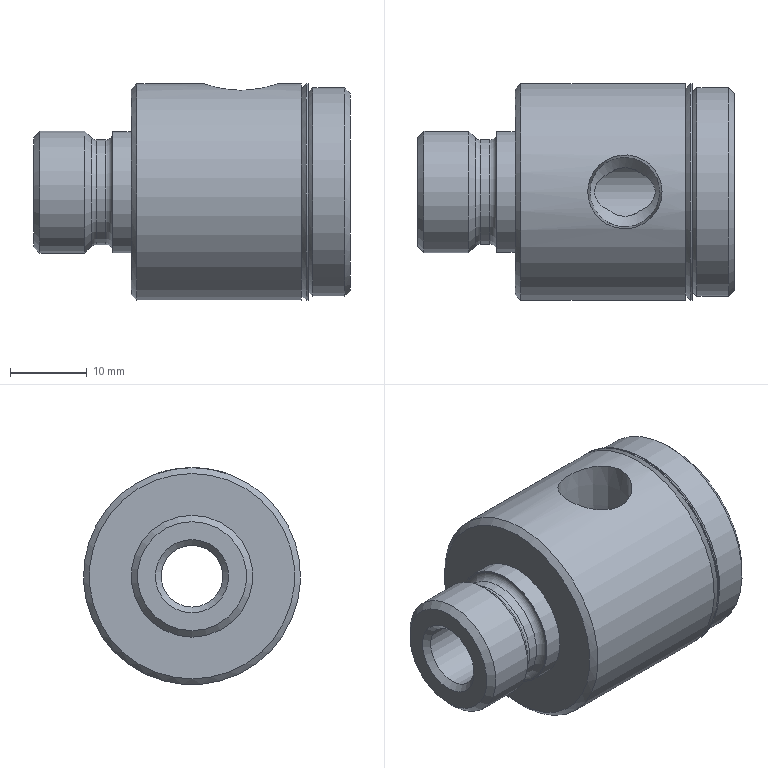Part | NX | features solid 2 | 1 solid | 30 faces | box 41.275 x 28.27 x 28.27 mm | volume 17100 mm3 | cone 11 | cylinder 10 | plane 6 | torus 3 | commonest cylinder face diameters 6.35 x2 28.27 x2 8.026 x1 13.678 x1 15.812 x1 15.875 x1
STEP:
#1=CARTESIAN_POINT('',(34.861,0.,14.135));
#2=VERTEX_POINT('',#1);
#3=CARTESIAN_POINT('',(34.861,0.,0.));
#4=DIRECTION('',(-1.,0.,0.));
#5=DIRECTION('',(0.,0.,1.));
#6=AXIS2_PLACEMENT_3D('',#3,#4,#5);
#7=CIRCLE('',#6,14.135);
#8=EDGE_CURVE('',#2,#2,#7,.T.);
#9=ORIENTED_EDGE('',*,*,#8,.F.);
#10=EDGE_LOOP('',(#9));
#11=FACE_BOUND('',#10,.T.);
#12=CARTESIAN_POINT('',(34.861,0.,13.449));
#13=VERTEX_POINT('',#12);
#14=CARTESIAN_POINT('',(34.861,0.,0.));
#15=DIRECTION('',(-1.,0.,0.));
#16=DIRECTION('',(0.,0.,1.));
#17=AXIS2_PLACEMENT_3D('',#14,#15,#16);
#18=CIRCLE('',#17,13.449);
#19=EDGE_CURVE('',#13,#13,#18,.T.);
#20=ORIENTED_EDGE('',*,*,#19,.T.);
#21=EDGE_LOOP('',(#20));
#22=FACE_BOUND('',#21,.T.);
#23=CARTESIAN_POINT('',(34.861,14.135,0.));
#24=DIRECTION('',(1.,0.,0.));
#25=DIRECTION('',(0.,0.,-1.));
#26=AXIS2_PLACEMENT_3D('',#23,#24,#25);
#27=PLANE('',#26);
#28=ADVANCED_FACE('',(#11,#22),#27,.T.);
#29=CARTESIAN_POINT('',(35.623,0.,12.846));
#30=VERTEX_POINT('',#29);
#31=CARTESIAN_POINT('',(35.623,0.,0.));
#32=DIRECTION('',(-1.,0.,0.));
#33=DIRECTION('',(0.,0.,1.));
#34=AXIS2_PLACEMENT_3D('',#31,#32,#33);
#35=CIRCLE('',#34,12.846);
#36=EDGE_CURVE('',#30,#30,#35,.T.);
#37=ORIENTED_EDGE('',*,*,#36,.T.);
#38=EDGE_LOOP('',(#37));
#39=FACE_BOUND('',#38,.T.);
#40=CARTESIAN_POINT('',(35.242,0.,12.846));
#41=VERTEX_POINT('',#40);
#42=CARTESIAN_POINT('',(35.242,0.,0.));
#43=DIRECTION('',(-1.,0.,0.));
#44=DIRECTION('',(0.,0.,1.));
#45=AXIS2_PLACEMENT_3D('',#42,#43,#44);
#46=CIRCLE('',#45,12.846);
#47=EDGE_CURVE('',#41,#41,#46,.T.);
#48=ORIENTED_EDGE('',*,*,#47,.F.);
#49=EDGE_LOOP('',(#48));
#50=FACE_BOUND('',#49,.T.);
#51=CARTESIAN_POINT('',(41.275,0.,0.));
#52=DIRECTION('',(-1.,0.,0.));
#53=DIRECTION('',(0.,0.,1.));
#54=AXIS2_PLACEMENT_3D('',#51,#52,#53);
#55=CYLINDRICAL_SURFACE('',#54,12.846);
#56=ADVANCED_FACE('',(#39,#50),#55,.T.);
#57=CARTESIAN_POINT('',(7.513,0.,7.099));
#58=VERTEX_POINT('',#57);
#59=CARTESIAN_POINT('',(7.513,0.,0.));
#60=DIRECTION('',(-1.,0.,0.));
#61=DIRECTION('',(0.,0.,1.));
#62=AXIS2_PLACEMENT_3D('',#59,#60,#61);
#63=CIRCLE('',#62,7.099);
#64=EDGE_CURVE('',#58,#58,#63,.T.);
#65=ORIENTED_EDGE('',*,*,#64,.T.);
#66=EDGE_LOOP('',(#65));
#67=FACE_BOUND('',#66,.T.);
#68=CARTESIAN_POINT('',(6.673,0.,7.938));
#69=VERTEX_POINT('',#68);
#70=CARTESIAN_POINT('',(6.673,0.,0.));
#71=DIRECTION('',(-1.,0.,0.));
#72=DIRECTION('',(0.,0.,1.));
#73=AXIS2_PLACEMENT_3D('',#70,#71,#72);
#74=CIRCLE('',#73,7.938);
#75=EDGE_CURVE('',#69,#69,#74,.T.);
#76=ORIENTED_EDGE('',*,*,#75,.F.);
#77=EDGE_LOOP('',(#76));
#78=FACE_BOUND('',#77,.T.);
#79=CARTESIAN_POINT('',(6.673,0.,0.));
#80=DIRECTION('',(-1.,0.,0.));
#81=DIRECTION('',(0.,0.,1.));
#82=AXIS2_PLACEMENT_3D('',#79,#80,#81);
#83=CONICAL_SURFACE('',#82,7.938,0.7846);
#84=ADVANCED_FACE('',(#67,#78),#83,.T.);
#85=ORIENTED_EDGE('',*,*,#64,.F.);
#86=EDGE_LOOP('',(#85));
#87=FACE_BOUND('',#86,.T.);
#88=CARTESIAN_POINT('',(8.141,0.,6.839));
#89=VERTEX_POINT('',#88);
#90=CARTESIAN_POINT('',(8.141,0.,0.));
#91=DIRECTION('',(-1.,0.,0.));
#92=DIRECTION('',(0.,0.,1.));
#93=AXIS2_PLACEMENT_3D('',#90,#91,#92);
#94=CIRCLE('',#93,6.839);
#95=EDGE_CURVE('',#89,#89,#94,.T.);
#96=ORIENTED_EDGE('',*,*,#95,.T.);
#97=EDGE_LOOP('',(#96));
#98=FACE_BOUND('',#97,.T.);
#99=CARTESIAN_POINT('',(8.141,0.,0.));
#100=DIRECTION('',(-1.,0.,0.));
#101=DIRECTION('',(0.,0.,1.));
#102=AXIS2_PLACEMENT_3D('',#99,#100,#101);
#103=TOROIDAL_SURFACE('',#102,7.728,0.889);
#104=ADVANCED_FACE('',(#87,#98),#103,.F.);
#105=CARTESIAN_POINT('',(9.423,0.,6.839));
#106=VERTEX_POINT('',#105);
#107=CARTESIAN_POINT('',(9.423,0.,0.));
#108=DIRECTION('',(-1.,0.,0.));
#109=DIRECTION('',(0.,0.,1.));
#110=AXIS2_PLACEMENT_3D('',#107,#108,#109);
#111=CIRCLE('',#110,6.839);
#112=EDGE_CURVE('',#106,#106,#111,.T.);
#113=ORIENTED_EDGE('',*,*,#112,.T.);
#114=EDGE_LOOP('',(#113));
#115=FACE_BOUND('',#114,.T.);
#116=ORIENTED_EDGE('',*,*,#95,.F.);
#117=EDGE_LOOP('',(#116));
#118=FACE_BOUND('',#117,.T.);
#119=CARTESIAN_POINT('',(12.7,0.,0.));
#120=DIRECTION('',(-1.,0.,0.));
#121=DIRECTION('',(0.,0.,1.));
#122=AXIS2_PLACEMENT_3D('',#119,#120,#121);
#123=CYLINDRICAL_SURFACE('',#122,6.839);
#124=ADVANCED_FACE('',(#115,#118),#123,.T.);
#125=ORIENTED_EDGE('',*,*,#112,.F.);
#126=EDGE_LOOP('',(#125));
#127=FACE_BOUND('',#126,.T.);
#128=CARTESIAN_POINT('',(10.312,0.,7.728));
#129=VERTEX_POINT('',#128);
#130=CARTESIAN_POINT('',(10.312,0.,0.));
#131=DIRECTION('',(-1.,0.,0.));
#132=DIRECTION('',(0.,0.,1.));
#133=AXIS2_PLACEMENT_3D('',#130,#131,#132);
#134=CIRCLE('',#133,7.728);
#135=EDGE_CURVE('',#129,#129,#134,.T.);
#136=ORIENTED_EDGE('',*,*,#135,.T.);
#137=EDGE_LOOP('',(#136));
#138=FACE_BOUND('',#137,.T.);
#139=CARTESIAN_POINT('',(9.423,0.,0.));
#140=DIRECTION('',(-1.,0.,0.));
#141=DIRECTION('',(0.,0.,1.));
#142=AXIS2_PLACEMENT_3D('',#139,#140,#141);
#143=TOROIDAL_SURFACE('',#142,7.728,0.889);
#144=ADVANCED_FACE('',(#127,#138),#143,.F.);
#145=CARTESIAN_POINT('',(10.312,0.,7.906));
#146=VERTEX_POINT('',#145);
#147=CARTESIAN_POINT('',(10.312,0.,0.));
#148=DIRECTION('',(-1.,0.,0.));
#149=DIRECTION('',(0.,0.,1.));
#150=AXIS2_PLACEMENT_3D('',#147,#148,#149);
#151=CIRCLE('',#150,7.906);
#152=EDGE_CURVE('',#146,#146,#151,.T.);
#153=ORIENTED_EDGE('',*,*,#152,.T.);
#154=EDGE_LOOP('',(#153));
#155=FACE_BOUND('',#154,.T.);
#156=ORIENTED_EDGE('',*,*,#135,.F.);
#157=EDGE_LOOP('',(#156));
#158=FACE_BOUND('',#157,.T.);
#159=CARTESIAN_POINT('',(10.312,7.728,0.));
#160=DIRECTION('',(-1.,0.,0.));
#161=DIRECTION('',(0.,0.,1.));
#162=AXIS2_PLACEMENT_3D('',#159,#160,#161);
#163=PLANE('',#162);
#164=ADVANCED_FACE('',(#155,#158),#163,.T.);
#165=CARTESIAN_POINT('',(12.7,0.,7.906));
#166=VERTEX_POINT('',#165);
#167=CARTESIAN_POINT('',(12.7,0.,0.));
#168=DIRECTION('',(-1.,0.,0.));
#169=DIRECTION('',(0.,0.,1.));
#170=AXIS2_PLACEMENT_3D('',#167,#168,#169);
#171=CIRCLE('',#170,7.906);
#172=EDGE_CURVE('',#166,#166,#171,.F.);
#173=ORIENTED_EDGE('',*,*,#172,.F.);
#174=EDGE_LOOP('',(#173));
#175=FACE_BOUND('',#174,.T.);
#176=ORIENTED_EDGE('',*,*,#152,.F.);
#177=EDGE_LOOP('',(#176));
#178=FACE_BOUND('',#177,.T.);
#179=CARTESIAN_POINT('',(12.7,0.,0.));
#180=DIRECTION('',(-1.,0.,0.));
#181=DIRECTION('',(0.,0.,1.));
#182=AXIS2_PLACEMENT_3D('',#179,#180,#181);
#183=CYLINDRICAL_SURFACE('',#182,7.906);
#184=ADVANCED_FACE('',(#175,#178),#183,.T.);
#185=CARTESIAN_POINT('',(0.,0.,-4.775));
#186=VERTEX_POINT('',#185);
#187=CARTESIAN_POINT('',(0.,0.,0.));
#188=DIRECTION('',(1.,0.,0.));
#189=DIRECTION('',(0.,0.,-1.));
#190=AXIS2_PLACEMENT_3D('',#187,#188,#189);
#191=CIRCLE('',#190,4.775);
#192=EDGE_CURVE('',#186,#186,#191,.T.);
#193=ORIENTED_EDGE('',*,*,#192,.T.);
#194=EDGE_LOOP('',(#193));
#195=FACE_BOUND('',#194,.T.);
#196=CARTESIAN_POINT('',(0.,0.,7.098));
#197=VERTEX_POINT('',#196);
#198=CARTESIAN_POINT('',(0.,0.,0.));
#199=DIRECTION('',(-1.,0.,0.));
#200=DIRECTION('',(0.,0.,1.));
#201=AXIS2_PLACEMENT_3D('',#198,#199,#200);
#202=CIRCLE('',#201,7.098);
#203=EDGE_CURVE('',#197,#197,#202,.T.);
#204=ORIENTED_EDGE('',*,*,#203,.T.);
#205=EDGE_LOOP('',(#204));
#206=FACE_BOUND('',#205,.T.);
#207=CARTESIAN_POINT('',(0.,0.,0.));
#208=DIRECTION('',(-1.,0.,0.));
#209=DIRECTION('',(0.,0.,1.));
#210=AXIS2_PLACEMENT_3D('',#207,#208,#209);
#211=PLANE('',#210);
#212=ADVANCED_FACE('',(#195,#206),#211,.T.);
#213=CARTESIAN_POINT('',(0.8395,0.,7.938));
#214=VERTEX_POINT('',#213);
#215=CARTESIAN_POINT('',(0.8395,0.,0.));
#216=DIRECTION('',(-1.,0.,0.));
#217=DIRECTION('',(0.,0.,1.));
#218=AXIS2_PLACEMENT_3D('',#215,#216,#217);
#219=CIRCLE('',#218,7.938);
#220=EDGE_CURVE('',#214,#214,#219,.T.);
#221=ORIENTED_EDGE('',*,*,#220,.T.);
#222=EDGE_LOOP('',(#221));
#223=FACE_BOUND('',#222,.T.);
#224=ORIENTED_EDGE('',*,*,#203,.F.);
#225=EDGE_LOOP('',(#224));
#226=FACE_BOUND('',#225,.T.);
#227=CARTESIAN_POINT('',(0.,0.,0.));
#228=DIRECTION('',(1.,0.,0.));
#229=DIRECTION('',(0.,0.,-1.));
#230=AXIS2_PLACEMENT_3D('',#227,#228,#229);
#231=CONICAL_SURFACE('',#230,7.098,0.7854);
#232=ADVANCED_FACE('',(#223,#226),#231,.T.);
#233=ORIENTED_EDGE('',*,*,#75,.T.);
#234=EDGE_LOOP('',(#233));
#235=FACE_BOUND('',#234,.T.);
#236=ORIENTED_EDGE('',*,*,#220,.F.);
#237=EDGE_LOOP('',(#236));
#238=FACE_BOUND('',#237,.T.);
#239=CARTESIAN_POINT('',(12.7,0.,0.));
#240=DIRECTION('',(-1.,0.,0.));
#241=DIRECTION('',(0.,0.,1.));
#242=AXIS2_PLACEMENT_3D('',#239,#240,#241);
#243=CYLINDRICAL_SURFACE('',#242,7.938);
#244=ADVANCED_FACE('',(#235,#238),#243,.T.);
#245=CARTESIAN_POINT('',(36.386,0.,13.608));
#246=VERTEX_POINT('',#245);
#247=CARTESIAN_POINT('',(36.386,0.,0.));
#248=DIRECTION('',(-1.,0.,0.));
#249=DIRECTION('',(0.,0.,1.));
#250=AXIS2_PLACEMENT_3D('',#247,#248,#249);
#251=CIRCLE('',#250,13.608);
#252=EDGE_CURVE('',#246,#246,#251,.T.);
#253=ORIENTED_EDGE('',*,*,#252,.T.);
#254=EDGE_LOOP('',(#253));
#255=FACE_BOUND('',#254,.T.);
#256=ORIENTED_EDGE('',*,*,#36,.F.);
#257=EDGE_LOOP('',(#256));
#258=FACE_BOUND('',#257,.T.);
#259=CARTESIAN_POINT('',(35.623,0.,0.));
#260=DIRECTION('',(1.,0.,0.));
#261=DIRECTION('',(0.,0.,-1.));
#262=AXIS2_PLACEMENT_3D('',#259,#260,#261);
#263=CONICAL_SURFACE('',#262,12.846,0.7854);
#264=ADVANCED_FACE('',(#255,#258),#263,.T.);
#265=CARTESIAN_POINT('',(40.513,0.,13.608));
#266=VERTEX_POINT('',#265);
#267=CARTESIAN_POINT('',(40.513,0.,0.));
#268=DIRECTION('',(-1.,0.,0.));
#269=DIRECTION('',(0.,0.,1.));
#270=AXIS2_PLACEMENT_3D('',#267,#268,#269);
#271=CIRCLE('',#270,13.608);
#272=EDGE_CURVE('',#266,#266,#271,.T.);
#273=ORIENTED_EDGE('',*,*,#272,.T.);
#274=EDGE_LOOP('',(#273));
#275=FACE_BOUND('',#274,.T.);
#276=ORIENTED_EDGE('',*,*,#252,.F.);
#277=EDGE_LOOP('',(#276));
#278=FACE_BOUND('',#277,.T.);
#279=CARTESIAN_POINT('',(41.275,0.,0.));
#280=DIRECTION('',(-1.,0.,0.));
#281=DIRECTION('',(0.,0.,1.));
#282=AXIS2_PLACEMENT_3D('',#279,#280,#281);
#283=CYLINDRICAL_SURFACE('',#282,13.608);
#284=ADVANCED_FACE('',(#275,#278),#283,.T.);
#285=CARTESIAN_POINT('',(41.275,0.,12.846));
#286=VERTEX_POINT('',#285);
#287=CARTESIAN_POINT('',(41.275,0.,0.));
#288=DIRECTION('',(-1.,0.,0.));
#289=DIRECTION('',(0.,0.,1.));
#290=AXIS2_PLACEMENT_3D('',#287,#288,#289);
#291=CIRCLE('',#290,12.846);
#292=EDGE_CURVE('',#286,#286,#291,.T.);
#293=ORIENTED_EDGE('',*,*,#292,.T.);
#294=EDGE_LOOP('',(#293));
#295=FACE_BOUND('',#294,.T.);
#296=ORIENTED_EDGE('',*,*,#272,.F.);
#297=EDGE_LOOP('',(#296));
#298=FACE_BOUND('',#297,.T.);
#299=CARTESIAN_POINT('',(40.513,0.,0.));
#300=DIRECTION('',(-1.,0.,0.));
#301=DIRECTION('',(0.,0.,1.));
#302=AXIS2_PLACEMENT_3D('',#299,#300,#301);
#303=CONICAL_SURFACE('',#302,13.608,0.7854);
#304=ADVANCED_FACE('',(#295,#298),#303,.T.);
#305=CARTESIAN_POINT('',(41.275,0.,-4.013));
#306=VERTEX_POINT('',#305);
#307=CARTESIAN_POINT('',(41.275,0.,0.));
#308=DIRECTION('',(1.,0.,0.));
#309=DIRECTION('',(0.,0.,-1.));
#310=AXIS2_PLACEMENT_3D('',#307,#308,#309);
#311=CIRCLE('',#310,4.013);
#312=EDGE_CURVE('',#306,#306,#311,.T.);
#313=ORIENTED_EDGE('',*,*,#312,.F.);
#314=EDGE_LOOP('',(#313));
#315=FACE_BOUND('',#314,.T.);
#316=ORIENTED_EDGE('',*,*,#292,.F.);
#317=EDGE_LOOP('',(#316));
#318=FACE_BOUND('',#317,.T.);
#319=CARTESIAN_POINT('',(41.275,12.846,0.));
#320=DIRECTION('',(1.,0.,0.));
#321=DIRECTION('',(0.,0.,-1.));
#322=AXIS2_PLACEMENT_3D('',#319,#320,#321);
#323=PLANE('',#322);
#324=ADVANCED_FACE('',(#315,#318),#323,.T.);
#325=ORIENTED_EDGE('',*,*,#172,.T.);
#326=EDGE_LOOP('',(#325));
#327=FACE_BOUND('',#326,.T.);
#328=CARTESIAN_POINT('',(12.7,0.,13.373));
#329=VERTEX_POINT('',#328);
#330=CARTESIAN_POINT('',(12.7,0.,0.));
#331=DIRECTION('',(-1.,0.,0.));
#332=DIRECTION('',(0.,0.,1.));
#333=AXIS2_PLACEMENT_3D('',#330,#331,#332);
#334=CIRCLE('',#333,13.373);
#335=EDGE_CURVE('',#329,#329,#334,.T.);
#336=ORIENTED_EDGE('',*,*,#335,.T.);
#337=EDGE_LOOP('',(#336));
#338=FACE_BOUND('',#337,.T.);
#339=CARTESIAN_POINT('',(12.7,0.,0.));
#340=DIRECTION('',(-1.,0.,0.));
#341=DIRECTION('',(0.,0.,1.));
#342=AXIS2_PLACEMENT_3D('',#339,#340,#341);
#343=PLANE('',#342);
#344=ADVANCED_FACE('',(#327,#338),#343,.T.);
#345=CARTESIAN_POINT('',(13.462,0.,14.135));
#346=VERTEX_POINT('',#345);
#347=CARTESIAN_POINT('',(13.462,0.,0.));
#348=DIRECTION('',(-1.,0.,0.));
#349=DIRECTION('',(0.,0.,1.));
#350=AXIS2_PLACEMENT_3D('',#347,#348,#349);
#351=CIRCLE('',#350,14.135);
#352=EDGE_CURVE('',#346,#346,#351,.T.);
#353=ORIENTED_EDGE('',*,*,#352,.T.);
#354=EDGE_LOOP('',(#353));
#355=FACE_BOUND('',#354,.T.);
#356=ORIENTED_EDGE('',*,*,#335,.F.);
#357=EDGE_LOOP('',(#356));
#358=FACE_BOUND('',#357,.T.);
#359=CARTESIAN_POINT('',(12.7,0.,0.));
#360=DIRECTION('',(1.,0.,0.));
#361=DIRECTION('',(0.,0.,-1.));
#362=AXIS2_PLACEMENT_3D('',#359,#360,#361);
#363=CONICAL_SURFACE('',#362,13.373,0.7854);
#364=ADVANCED_FACE('',(#355,#358),#363,.T.);
#365=CARTESIAN_POINT('',(23.692,-3.513,13.691));
#366=VERTEX_POINT('',#365);
#367=CARTESIAN_POINT('',(21.636,-0.1674,14.34));
#368=CARTESIAN_POINT('',(23.337,-3.897,13.683));
#369=CARTESIAN_POINT('',(27.171,-5.326,13.076));
#370=CARTESIAN_POINT('',(30.898,-3.664,13.762));
#371=CARTESIAN_POINT('',(32.366,0.1695,14.34));
#372=CARTESIAN_POINT('',(30.663,3.895,13.684));
#373=CARTESIAN_POINT('',(26.836,5.328,13.075));
#374=CARTESIAN_POINT('',(23.097,3.659,13.763));
#375=CARTESIAN_POINT('',(21.636,-0.1674,14.34));
#376=CARTESIAN_POINT('',(23.337,-3.897,13.683));
#377=CARTESIAN_POINT('',(27.171,-5.326,13.076));
#378=B_SPLINE_CURVE_WITH_KNOTS('',3,(#367,#368,#369,#370,#371,#372,#373,#374,#375,#376,#377),.UNSPECIFIED.,.T.,.F.,(1,1,1,1,1,1,1,1,1,1,1,1,1,1,1),(-0.0114,-0.007602,-0.003801,0.,0.003801,0.007602,0.0114,0.0152,0.01901,0.02281,0.02661,0.03041,0.03421,0.03801,0.04181),.UNSPECIFIED.);
#379=EDGE_CURVE('',#366,#366,#378,.T.);
#380=ORIENTED_EDGE('',*,*,#379,.F.);
#381=EDGE_LOOP('',(#380));
#382=FACE_BOUND('',#381,.T.);
#383=ORIENTED_EDGE('',*,*,#8,.T.);
#384=EDGE_LOOP('',(#383));
#385=FACE_BOUND('',#384,.T.);
#386=ORIENTED_EDGE('',*,*,#352,.F.);
#387=EDGE_LOOP('',(#386));
#388=FACE_BOUND('',#387,.T.);
#389=CARTESIAN_POINT('',(41.275,0.,0.));
#390=DIRECTION('',(-1.,0.,0.));
#391=DIRECTION('',(0.,0.,1.));
#392=AXIS2_PLACEMENT_3D('',#389,#390,#391);
#393=CYLINDRICAL_SURFACE('',#392,14.135);
#394=ADVANCED_FACE('',(#382,#385,#388),#393,.T.);
#395=CARTESIAN_POINT('',(24.881,-2.364,3.243));
#396=VERTEX_POINT('',#395);
#397=CARTESIAN_POINT('',(29.12,-2.364,3.243));
#398=VERTEX_POINT('',#397);
#399=CARTESIAN_POINT('',(24.881,-2.364,3.243));
#400=CARTESIAN_POINT('',(25.158,-2.613,3.062));
#401=CARTESIAN_POINT('',(25.778,-3.006,2.683));
#402=CARTESIAN_POINT('',(26.997,-3.259,2.341));
#403=CARTESIAN_POINT('',(28.22,-3.008,2.682));
#404=CARTESIAN_POINT('',(28.842,-2.613,3.062));
#405=CARTESIAN_POINT('',(29.12,-2.364,3.243));
#406=B_SPLINE_CURVE_WITH_KNOTS('',3,(#399,#400,#401,#402,#403,#404,#405),.UNSPECIFIED.,.F.,.F.,(4,1,1,1,4),(0.,0.001229,0.002458,0.003687,0.004916),.UNSPECIFIED.);
#407=EDGE_CURVE('',#396,#398,#406,.T.);
#408=ORIENTED_EDGE('',*,*,#407,.T.);
#409=CARTESIAN_POINT('',(29.12,2.364,3.243));
#410=VERTEX_POINT('',#409);
#411=CARTESIAN_POINT('',(29.12,-2.364,3.243));
#412=CARTESIAN_POINT('',(29.592,-2.15,3.399));
#413=CARTESIAN_POINT('',(30.461,-1.586,3.768));
#414=CARTESIAN_POINT('',(31.186,-0.005228,4.135));
#415=CARTESIAN_POINT('',(30.466,1.582,3.77));
#416=CARTESIAN_POINT('',(29.596,2.148,3.4));
#417=CARTESIAN_POINT('',(29.12,2.364,3.243));
#418=B_SPLINE_CURVE_WITH_KNOTS('',3,(#411,#412,#413,#414,#415,#416,#417),.UNSPECIFIED.,.F.,.F.,(4,1,1,1,4),(0.000274,0.00189,0.003505,0.005121,0.006736),.UNSPECIFIED.);
#419=EDGE_CURVE('',#398,#410,#418,.T.);
#420=ORIENTED_EDGE('',*,*,#419,.T.);
#421=CARTESIAN_POINT('',(24.881,2.364,3.243));
#422=VERTEX_POINT('',#421);
#423=CARTESIAN_POINT('',(29.12,2.364,3.243));
#424=CARTESIAN_POINT('',(28.842,2.613,3.062));
#425=CARTESIAN_POINT('',(28.222,3.006,2.683));
#426=CARTESIAN_POINT('',(27.004,3.259,2.341));
#427=CARTESIAN_POINT('',(25.78,3.008,2.682));
#428=CARTESIAN_POINT('',(25.158,2.613,3.062));
#429=CARTESIAN_POINT('',(24.881,2.364,3.243));
#430=B_SPLINE_CURVE_WITH_KNOTS('',3,(#423,#424,#425,#426,#427,#428,#429),.UNSPECIFIED.,.F.,.F.,(4,1,1,1,4),(0.,0.001229,0.002458,0.003687,0.004916),.UNSPECIFIED.);
#431=EDGE_CURVE('',#410,#422,#430,.T.);
#432=ORIENTED_EDGE('',*,*,#431,.T.);
#433=CARTESIAN_POINT('',(24.881,2.364,3.243));
#434=CARTESIAN_POINT('',(24.408,2.15,3.399));
#435=CARTESIAN_POINT('',(23.538,1.585,3.768));
#436=CARTESIAN_POINT('',(22.814,0.003901,4.135));
#437=CARTESIAN_POINT('',(23.534,-1.583,3.77));
#438=CARTESIAN_POINT('',(24.409,-2.15,3.399));
#439=CARTESIAN_POINT('',(24.881,-2.364,3.243));
#440=B_SPLINE_CURVE_WITH_KNOTS('',3,(#433,#434,#435,#436,#437,#438,#439),.UNSPECIFIED.,.F.,.F.,(4,1,1,1,4),(0.01114,0.01276,0.01437,0.01599,0.0176),.UNSPECIFIED.);
#441=EDGE_CURVE('',#422,#396,#440,.T.);
#442=ORIENTED_EDGE('',*,*,#441,.T.);
#443=EDGE_LOOP('',(#408,#420,#432,#442));
#444=FACE_BOUND('',#443,.T.);
#445=ORIENTED_EDGE('',*,*,#312,.T.);
#446=EDGE_LOOP('',(#445));
#447=FACE_BOUND('',#446,.T.);
#448=CARTESIAN_POINT('',(0.762,0.,-4.013));
#449=VERTEX_POINT('',#448);
#450=CARTESIAN_POINT('',(0.762,0.,0.));
#451=DIRECTION('',(1.,0.,0.));
#452=DIRECTION('',(0.,0.,-1.));
#453=AXIS2_PLACEMENT_3D('',#450,#451,#452);
#454=CIRCLE('',#453,4.013);
#455=EDGE_CURVE('',#449,#449,#454,.T.);
#456=ORIENTED_EDGE('',*,*,#455,.F.);
#457=EDGE_LOOP('',(#456));
#458=FACE_BOUND('',#457,.T.);
#459=CARTESIAN_POINT('',(41.275,0.,0.));
#460=DIRECTION('',(1.,0.,0.));
#461=DIRECTION('',(0.,0.,-1.));
#462=AXIS2_PLACEMENT_3D('',#459,#460,#461);
#463=CYLINDRICAL_SURFACE('',#462,4.013);
#464=ADVANCED_FACE('',(#444,#447,#458),#463,.F.);
#465=ORIENTED_EDGE('',*,*,#455,.T.);
#466=EDGE_LOOP('',(#465));
#467=FACE_BOUND('',#466,.T.);
#468=ORIENTED_EDGE('',*,*,#192,.F.);
#469=EDGE_LOOP('',(#468));
#470=FACE_BOUND('',#469,.T.);
#471=CARTESIAN_POINT('',(0.,0.,0.));
#472=DIRECTION('',(-1.,0.,0.));
#473=DIRECTION('',(0.,0.,1.));
#474=AXIS2_PLACEMENT_3D('',#471,#472,#473);
#475=CONICAL_SURFACE('',#474,4.775,0.7854);
#476=ADVANCED_FACE('',(#467,#470),#475,.F.);
#477=CARTESIAN_POINT('',(27.,0.,3.243));
#478=DIRECTION('',(0.,0.,-1.));
#479=DIRECTION('',(-1.,0.,0.));
#480=AXIS2_PLACEMENT_3D('',#477,#478,#479);
#481=CIRCLE('',#480,3.175);
#482=EDGE_CURVE('',#422,#410,#481,.T.);
#483=ORIENTED_EDGE('',*,*,#482,.F.);
#484=ORIENTED_EDGE('',*,*,#431,.F.);
#485=EDGE_LOOP('',(#483,#484));
#486=FACE_BOUND('',#485,.T.);
#487=CARTESIAN_POINT('',(27.,0.,14.135));
#488=DIRECTION('',(0.,0.,-1.));
#489=DIRECTION('',(-1.,0.,0.));
#490=AXIS2_PLACEMENT_3D('',#487,#488,#489);
#491=CYLINDRICAL_SURFACE('',#490,3.175);
#492=ADVANCED_FACE('',(#486),#491,.F.);
#493=CARTESIAN_POINT('',(27.,0.,3.243));
#494=DIRECTION('',(0.,0.,-1.));
#495=DIRECTION('',(-1.,0.,0.));
#496=AXIS2_PLACEMENT_3D('',#493,#494,#495);
#497=CIRCLE('',#496,3.175);
#498=EDGE_CURVE('',#398,#396,#497,.T.);
#499=ORIENTED_EDGE('',*,*,#498,.F.);
#500=ORIENTED_EDGE('',*,*,#407,.F.);
#501=EDGE_LOOP('',(#499,#500));
#502=FACE_BOUND('',#501,.T.);
#503=CARTESIAN_POINT('',(27.,0.,14.135));
#504=DIRECTION('',(0.,0.,-1.));
#505=DIRECTION('',(-1.,0.,0.));
#506=AXIS2_PLACEMENT_3D('',#503,#504,#505);
#507=CYLINDRICAL_SURFACE('',#506,3.175);
#508=ADVANCED_FACE('',(#502),#507,.F.);
#509=CARTESIAN_POINT('',(22.458,0.,4.61));
#510=VERTEX_POINT('',#509);
#511=CARTESIAN_POINT('',(27.,0.,4.61));
#512=DIRECTION('',(0.,0.,-1.));
#513=DIRECTION('',(-1.,0.,0.));
#514=AXIS2_PLACEMENT_3D('',#511,#512,#513);
#515=CIRCLE('',#514,4.542);
#516=EDGE_CURVE('',#510,#510,#515,.T.);
#517=ORIENTED_EDGE('',*,*,#516,.F.);
#518=EDGE_LOOP('',(#517));
#519=FACE_BOUND('',#518,.T.);
#520=ORIENTED_EDGE('',*,*,#498,.T.);
#521=ORIENTED_EDGE('',*,*,#441,.F.);
#522=ORIENTED_EDGE('',*,*,#482,.T.);
#523=ORIENTED_EDGE('',*,*,#419,.F.);
#524=EDGE_LOOP('',(#520,#521,#522,#523));
#525=FACE_BOUND('',#524,.T.);
#526=CARTESIAN_POINT('',(27.,0.,3.243));
#527=DIRECTION('',(0.,0.,1.));
#528=DIRECTION('',(1.,0.,0.));
#529=AXIS2_PLACEMENT_3D('',#526,#527,#528);
#530=CONICAL_SURFACE('',#529,3.175,0.7854);
#531=ADVANCED_FACE('',(#519,#525),#530,.F.);
#532=ORIENTED_EDGE('',*,*,#379,.T.);
#533=EDGE_LOOP('',(#532));
#534=FACE_BOUND('',#533,.T.);
#535=ORIENTED_EDGE('',*,*,#516,.T.);
#536=EDGE_LOOP('',(#535));
#537=FACE_BOUND('',#536,.T.);
#538=CARTESIAN_POINT('',(27.,0.,4.61));
#539=DIRECTION('',(0.,0.,1.));
#540=DIRECTION('',(1.,0.,0.));
#541=AXIS2_PLACEMENT_3D('',#538,#539,#540);
#542=CONICAL_SURFACE('',#541,4.542,0.03121);
#543=ADVANCED_FACE('',(#534,#537),#542,.F.);
#544=CARTESIAN_POINT('',(35.548,0.,14.135));
#545=VERTEX_POINT('',#544);
#546=CARTESIAN_POINT('',(35.548,0.,0.));
#547=DIRECTION('',(-1.,0.,0.));
#548=DIRECTION('',(0.,0.,1.));
#549=AXIS2_PLACEMENT_3D('',#546,#547,#548);
#550=CIRCLE('',#549,14.135);
#551=EDGE_CURVE('',#545,#545,#550,.T.);
#552=ORIENTED_EDGE('',*,*,#551,.F.);
#553=EDGE_LOOP('',(#552));
#554=FACE_BOUND('',#553,.T.);
#555=CARTESIAN_POINT('',(35.751,0.,14.135));
#556=VERTEX_POINT('',#555);
#557=CARTESIAN_POINT('',(35.751,0.,0.));
#558=DIRECTION('',(-1.,0.,0.));
#559=DIRECTION('',(0.,0.,1.));
#560=AXIS2_PLACEMENT_3D('',#557,#558,#559);
#561=CIRCLE('',#560,14.135);
#562=EDGE_CURVE('',#556,#556,#561,.T.);
#563=ORIENTED_EDGE('',*,*,#562,.T.);
#564=EDGE_LOOP('',(#563));
#565=FACE_BOUND('',#564,.T.);
#566=CARTESIAN_POINT('',(35.623,0.,0.));
#567=DIRECTION('',(-1.,0.,0.));
#568=DIRECTION('',(0.,0.,1.));
#569=AXIS2_PLACEMENT_3D('',#566,#567,#568);
#570=CYLINDRICAL_SURFACE('',#569,14.135);
#571=ADVANCED_FACE('',(#554,#565),#570,.T.);
#572=ORIENTED_EDGE('',*,*,#19,.F.);
#573=EDGE_LOOP('',(#572));
#574=FACE_BOUND('',#573,.T.);
#575=ORIENTED_EDGE('',*,*,#551,.T.);
#576=EDGE_LOOP('',(#575));
#577=FACE_BOUND('',#576,.T.);
#578=CARTESIAN_POINT('',(35.548,0.,0.));
#579=DIRECTION('',(1.,0.,0.));
#580=DIRECTION('',(0.,0.,-1.));
#581=AXIS2_PLACEMENT_3D('',#578,#579,#580);
#582=CONICAL_SURFACE('',#581,14.135,0.7854);
#583=ADVANCED_FACE('',(#574,#577),#582,.T.);
#584=CARTESIAN_POINT('',(34.984,0.,13.105));
#585=VERTEX_POINT('',#584);
#586=CARTESIAN_POINT('',(34.984,0.,0.));
#587=DIRECTION('',(-1.,0.,0.));
#588=DIRECTION('',(0.,0.,1.));
#589=AXIS2_PLACEMENT_3D('',#586,#587,#588);
#590=CIRCLE('',#589,13.105);
#591=EDGE_CURVE('',#585,#585,#590,.T.);
#592=ORIENTED_EDGE('',*,*,#591,.F.);
#593=EDGE_LOOP('',(#592));
#594=FACE_BOUND('',#593,.T.);
#595=ORIENTED_EDGE('',*,*,#47,.T.);
#596=EDGE_LOOP('',(#595));
#597=FACE_BOUND('',#596,.T.);
#598=CARTESIAN_POINT('',(35.242,0.,0.));
#599=DIRECTION('',(-1.,0.,0.));
#600=DIRECTION('',(0.,0.,1.));
#601=AXIS2_PLACEMENT_3D('',#598,#599,#600);
#602=CONICAL_SURFACE('',#601,12.846,0.7854);
#603=ADVANCED_FACE('',(#594,#597),#602,.T.);
#604=ORIENTED_EDGE('',*,*,#591,.T.);
#605=EDGE_LOOP('',(#604));
#606=FACE_BOUND('',#605,.T.);
#607=CARTESIAN_POINT('',(34.984,0.,13.284));
#608=VERTEX_POINT('',#607);
#609=CARTESIAN_POINT('',(34.984,0.,0.));
#610=DIRECTION('',(-1.,0.,0.));
#611=DIRECTION('',(0.,0.,1.));
#612=AXIS2_PLACEMENT_3D('',#609,#610,#611);
#613=CIRCLE('',#612,13.284);
#614=EDGE_CURVE('',#608,#608,#613,.T.);
#615=ORIENTED_EDGE('',*,*,#614,.F.);
#616=EDGE_LOOP('',(#615));
#617=FACE_BOUND('',#616,.T.);
#618=CARTESIAN_POINT('',(35.074,0.,0.));
#619=DIRECTION('',(-1.,0.,0.));
#620=DIRECTION('',(0.,0.,1.));
#621=AXIS2_PLACEMENT_3D('',#618,#619,#620);
#622=TOROIDAL_SURFACE('',#621,13.194,0.127);
#623=ADVANCED_FACE('',(#606,#617),#622,.F.);
#624=CARTESIAN_POINT('',(35.751,0.,14.051));
#625=VERTEX_POINT('',#624);
#626=CARTESIAN_POINT('',(35.751,0.,0.));
#627=DIRECTION('',(-1.,0.,0.));
#628=DIRECTION('',(0.,0.,1.));
#629=AXIS2_PLACEMENT_3D('',#626,#627,#628);
#630=CIRCLE('',#629,14.051);
#631=EDGE_CURVE('',#625,#625,#630,.T.);
#632=ORIENTED_EDGE('',*,*,#631,.F.);
#633=EDGE_LOOP('',(#632));
#634=FACE_BOUND('',#633,.T.);
#635=ORIENTED_EDGE('',*,*,#614,.T.);
#636=EDGE_LOOP('',(#635));
#637=FACE_BOUND('',#636,.T.);
#638=CARTESIAN_POINT('',(34.984,0.,0.));
#639=DIRECTION('',(1.,0.,0.));
#640=DIRECTION('',(0.,0.,-1.));
#641=AXIS2_PLACEMENT_3D('',#638,#639,#640);
#642=CONICAL_SURFACE('',#641,13.284,0.7854);
#643=ADVANCED_FACE('',(#634,#637),#642,.F.);
#644=ORIENTED_EDGE('',*,*,#562,.F.);
#645=EDGE_LOOP('',(#644));
#646=FACE_BOUND('',#645,.T.);
#647=ORIENTED_EDGE('',*,*,#631,.T.);
#648=EDGE_LOOP('',(#647));
#649=FACE_BOUND('',#648,.T.);
#650=CARTESIAN_POINT('',(35.751,14.051,0.));
#651=DIRECTION('',(-1.,0.,0.));
#652=DIRECTION('',(0.,0.,1.));
#653=AXIS2_PLACEMENT_3D('',#650,#651,#652);
#654=PLANE('',#653);
#655=ADVANCED_FACE('',(#646,#649),#654,.F.);
#656=CLOSED_SHELL('',(#28,#56,#84,#104,#124,#144,#164,#184,#212,#232,#244,#264,#284,#304,#324,#344,#364,#394,#464,#476,#492,#508,#531,#543,#571,#583,#603,#623,#643,#655));
#657=MANIFOLD_SOLID_BREP('',#656);
#658=(LENGTH_UNIT()NAMED_UNIT(*)SI_UNIT(.MILLI.,.METRE.));
#659=UNCERTAINTY_MEASURE_WITH_UNIT(LENGTH_MEASURE(0.0508),#658,'','');
#660=(NAMED_UNIT(*)PLANE_ANGLE_UNIT()SI_UNIT($,.RADIAN.));
#661=(NAMED_UNIT(*)SI_UNIT($,.STERADIAN.)SOLID_ANGLE_UNIT());
#662=(GEOMETRIC_REPRESENTATION_CONTEXT(3)GLOBAL_UNCERTAINTY_ASSIGNED_CONTEXT((#659))GLOBAL_UNIT_ASSIGNED_CONTEXT((#658,#660,#661))REPRESENTATION_CONTEXT('',''));
#663=ADVANCED_BREP_SHAPE_REPRESENTATION('',(#657),#662);